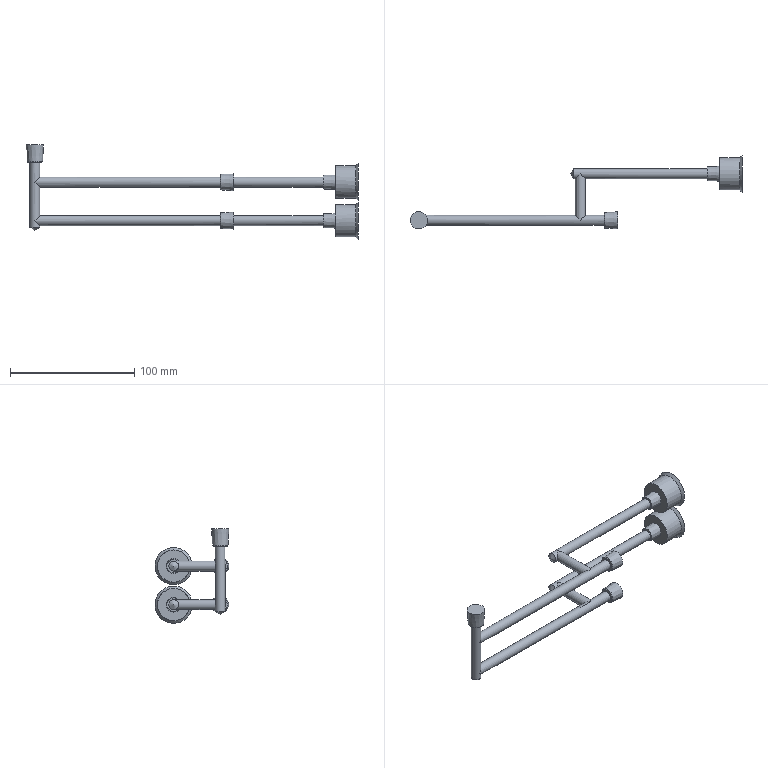Part | STEP file | COOLING-CAV_id202_x_t | 1 solid | 34 faces | box 267.068 x 59.568 x 76.003 mm | volume 57701 mm3 | cone 13 | plane 12 | cylinder 9 | commonest cylinder face diameters 8 x7 26 x2
STEP:
#1=CARTESIAN_POINT('',(200.,90.5,-11.));
#2=VERTEX_POINT('',#1);
#3=CARTESIAN_POINT('',(200.,75.5,-11.));
#4=DIRECTION('',(-1.,0.,0.));
#5=DIRECTION('',(0.,1.,0.));
#6=AXIS2_PLACEMENT_3D('',#3,#4,#5);
#7=CIRCLE('',#6,15.);
#8=EDGE_CURVE('',#2,#2,#7,.T.);
#9=ORIENTED_EDGE('',*,*,#8,.F.);
#10=EDGE_LOOP('',(#9));
#11=FACE_OUTER_BOUND('',#10,.T.);
#12=CARTESIAN_POINT('',(200.,75.5,-11.));
#13=DIRECTION('',(1.,0.,0.));
#14=DIRECTION('',(0.,0.,-1.));
#15=AXIS2_PLACEMENT_3D('',#12,#13,#14);
#16=PLANE('',#15);
#17=ADVANCED_FACE('',(#11),#16,.T.);
#18=ORIENTED_EDGE('',*,*,#8,.T.);
#19=EDGE_LOOP('',(#18));
#20=FACE_BOUND('',#19,.T.);
#21=CARTESIAN_POINT('',(198.,75.5,-24.));
#22=VERTEX_POINT('',#21);
#23=CARTESIAN_POINT('',(198.,75.5,-11.));
#24=DIRECTION('',(-1.,0.,0.));
#25=DIRECTION('',(0.,0.,-1.));
#26=AXIS2_PLACEMENT_3D('',#23,#24,#25);
#27=CIRCLE('',#26,13.);
#28=EDGE_CURVE('',#22,#22,#27,.T.);
#29=ORIENTED_EDGE('',*,*,#28,.F.);
#30=EDGE_LOOP('',(#29));
#31=FACE_BOUND('',#30,.T.);
#32=CARTESIAN_POINT('',(200.,75.5,-11.));
#33=DIRECTION('',(1.,0.,0.));
#34=DIRECTION('',(0.,1.,0.));
#35=AXIS2_PLACEMENT_3D('',#32,#33,#34);
#36=CONICAL_SURFACE('',#35,15.,45.);
#37=ADVANCED_FACE('',(#20,#31),#36,.T.);
#38=CARTESIAN_POINT('',(200.,90.5,20.));
#39=VERTEX_POINT('',#38);
#40=CARTESIAN_POINT('',(200.,75.5,20.));
#41=DIRECTION('',(-1.,0.,0.));
#42=DIRECTION('',(0.,1.,0.));
#43=AXIS2_PLACEMENT_3D('',#40,#41,#42);
#44=CIRCLE('',#43,15.);
#45=EDGE_CURVE('',#39,#39,#44,.T.);
#46=ORIENTED_EDGE('',*,*,#45,.F.);
#47=EDGE_LOOP('',(#46));
#48=FACE_OUTER_BOUND('',#47,.T.);
#49=CARTESIAN_POINT('',(200.,75.5,20.));
#50=DIRECTION('',(-1.,0.,0.));
#51=DIRECTION('',(0.,0.,1.));
#52=AXIS2_PLACEMENT_3D('',#49,#50,#51);
#53=PLANE('',#52);
#54=ADVANCED_FACE('',(#48),#53,.F.);
#55=ORIENTED_EDGE('',*,*,#28,.T.);
#56=EDGE_LOOP('',(#55));
#57=FACE_BOUND('',#56,.T.);
#58=CARTESIAN_POINT('',(182.001,75.5,-24.));
#59=VERTEX_POINT('',#58);
#60=CARTESIAN_POINT('',(182.001,75.5,-11.));
#61=DIRECTION('',(1.,0.,0.));
#62=DIRECTION('',(0.,0.,-1.));
#63=AXIS2_PLACEMENT_3D('',#60,#61,#62);
#64=CIRCLE('',#63,13.);
#65=EDGE_CURVE('',#59,#59,#64,.T.);
#66=ORIENTED_EDGE('',*,*,#65,.T.);
#67=EDGE_LOOP('',(#66));
#68=FACE_BOUND('',#67,.T.);
#69=CARTESIAN_POINT('',(206.888,75.5,-11.));
#70=DIRECTION('',(1.,0.,0.));
#71=DIRECTION('',(0.,0.,-1.));
#72=AXIS2_PLACEMENT_3D('',#69,#70,#71);
#73=CYLINDRICAL_SURFACE('',#72,13.);
#74=ADVANCED_FACE('',(#57,#68),#73,.T.);
#75=CARTESIAN_POINT('',(198.,75.5,33.));
#76=VERTEX_POINT('',#75);
#77=CARTESIAN_POINT('',(198.,75.5,20.));
#78=DIRECTION('',(-1.,0.,0.));
#79=DIRECTION('',(0.,0.,1.));
#80=AXIS2_PLACEMENT_3D('',#77,#78,#79);
#81=CIRCLE('',#80,13.);
#82=EDGE_CURVE('',#76,#76,#81,.T.);
#83=ORIENTED_EDGE('',*,*,#82,.F.);
#84=EDGE_LOOP('',(#83));
#85=FACE_BOUND('',#84,.T.);
#86=ORIENTED_EDGE('',*,*,#45,.T.);
#87=EDGE_LOOP('',(#86));
#88=FACE_BOUND('',#87,.T.);
#89=CARTESIAN_POINT('',(200.,75.5,20.));
#90=DIRECTION('',(1.,0.,0.));
#91=DIRECTION('',(0.,1.,0.));
#92=AXIS2_PLACEMENT_3D('',#89,#90,#91);
#93=CONICAL_SURFACE('',#92,15.,45.);
#94=ADVANCED_FACE('',(#85,#88),#93,.T.);
#95=CARTESIAN_POINT('',(182.001,75.5,-16.955));
#96=VERTEX_POINT('',#95);
#97=CARTESIAN_POINT('',(182.001,75.5,-11.));
#98=DIRECTION('',(-1.,0.,0.));
#99=DIRECTION('',(0.,0.,-1.));
#100=AXIS2_PLACEMENT_3D('',#97,#98,#99);
#101=CIRCLE('',#100,5.955);
#102=EDGE_CURVE('',#96,#96,#101,.T.);
#103=ORIENTED_EDGE('',*,*,#102,.F.);
#104=EDGE_LOOP('',(#103));
#105=FACE_BOUND('',#104,.T.);
#106=ORIENTED_EDGE('',*,*,#65,.F.);
#107=EDGE_LOOP('',(#106));
#108=FACE_BOUND('',#107,.T.);
#109=CARTESIAN_POINT('',(182.001,75.5,-11.));
#110=DIRECTION('',(1.,0.,0.));
#111=DIRECTION('',(0.,0.,-1.));
#112=AXIS2_PLACEMENT_3D('',#109,#110,#111);
#113=PLANE('',#112);
#114=ADVANCED_FACE('',(#105,#108),#113,.F.);
#115=CARTESIAN_POINT('',(182.001,75.5,33.));
#116=VERTEX_POINT('',#115);
#117=CARTESIAN_POINT('',(182.001,75.5,20.));
#118=DIRECTION('',(-1.,0.,0.));
#119=DIRECTION('',(0.,0.,1.));
#120=AXIS2_PLACEMENT_3D('',#117,#118,#119);
#121=CIRCLE('',#120,13.);
#122=EDGE_CURVE('',#116,#116,#121,.T.);
#123=ORIENTED_EDGE('',*,*,#122,.F.);
#124=EDGE_LOOP('',(#123));
#125=FACE_BOUND('',#124,.T.);
#126=ORIENTED_EDGE('',*,*,#82,.T.);
#127=EDGE_LOOP('',(#126));
#128=FACE_BOUND('',#127,.T.);
#129=CARTESIAN_POINT('',(55.348,75.5,20.));
#130=DIRECTION('',(-1.,0.,0.));
#131=DIRECTION('',(0.,0.,1.));
#132=AXIS2_PLACEMENT_3D('',#129,#130,#131);
#133=CYLINDRICAL_SURFACE('',#132,13.);
#134=ADVANCED_FACE('',(#125,#128),#133,.T.);
#135=ORIENTED_EDGE('',*,*,#102,.T.);
#136=EDGE_LOOP('',(#135));
#137=FACE_BOUND('',#136,.T.);
#138=CARTESIAN_POINT('',(172.001,75.5,-16.5));
#139=VERTEX_POINT('',#138);
#140=CARTESIAN_POINT('',(172.001,75.5,-11.));
#141=DIRECTION('',(1.,0.,0.));
#142=DIRECTION('',(0.,0.,-1.));
#143=AXIS2_PLACEMENT_3D('',#140,#141,#142);
#144=CIRCLE('',#143,5.5);
#145=EDGE_CURVE('',#139,#139,#144,.T.);
#146=ORIENTED_EDGE('',*,*,#145,.T.);
#147=EDGE_LOOP('',(#146));
#148=FACE_BOUND('',#147,.T.);
#149=CARTESIAN_POINT('',(182.001,75.5,-11.));
#150=DIRECTION('',(1.,0.,0.));
#151=DIRECTION('',(0.,0.,-1.));
#152=AXIS2_PLACEMENT_3D('',#149,#150,#151);
#153=CONICAL_SURFACE('',#152,5.955,2.603);
#154=ADVANCED_FACE('',(#137,#148),#153,.T.);
#155=CARTESIAN_POINT('',(182.001,75.5,14.045));
#156=VERTEX_POINT('',#155);
#157=CARTESIAN_POINT('',(182.001,75.5,20.));
#158=DIRECTION('',(-1.,0.,0.));
#159=DIRECTION('',(0.,0.,-1.));
#160=AXIS2_PLACEMENT_3D('',#157,#158,#159);
#161=CIRCLE('',#160,5.955);
#162=EDGE_CURVE('',#156,#156,#161,.T.);
#163=ORIENTED_EDGE('',*,*,#162,.F.);
#164=EDGE_LOOP('',(#163));
#165=FACE_BOUND('',#164,.T.);
#166=ORIENTED_EDGE('',*,*,#122,.T.);
#167=EDGE_LOOP('',(#166));
#168=FACE_BOUND('',#167,.T.);
#169=CARTESIAN_POINT('',(182.001,75.5,20.));
#170=DIRECTION('',(-1.,0.,0.));
#171=DIRECTION('',(0.,0.,1.));
#172=AXIS2_PLACEMENT_3D('',#169,#170,#171);
#173=PLANE('',#172);
#174=ADVANCED_FACE('',(#165,#168),#173,.T.);
#175=CARTESIAN_POINT('',(100.,44.884,-11.));
#176=VERTEX_POINT('',#175);
#177=CARTESIAN_POINT('',(100.,38.,-11.));
#178=DIRECTION('',(-1.,0.,0.));
#179=DIRECTION('',(0.,1.,0.));
#180=AXIS2_PLACEMENT_3D('',#177,#178,#179);
#181=CIRCLE('',#180,6.884);
#182=EDGE_CURVE('',#176,#176,#181,.T.);
#183=ORIENTED_EDGE('',*,*,#182,.F.);
#184=EDGE_LOOP('',(#183));
#185=FACE_OUTER_BOUND('',#184,.T.);
#186=CARTESIAN_POINT('',(100.,38.,-11.));
#187=DIRECTION('',(1.,0.,0.));
#188=DIRECTION('',(0.,0.,-1.));
#189=AXIS2_PLACEMENT_3D('',#186,#187,#188);
#190=PLANE('',#189);
#191=ADVANCED_FACE('',(#185),#190,.T.);
#192=CARTESIAN_POINT('',(172.001,75.5,-15.));
#193=VERTEX_POINT('',#192);
#194=CARTESIAN_POINT('',(172.001,75.5,-11.));
#195=DIRECTION('',(-1.,0.,0.));
#196=DIRECTION('',(0.,0.,-1.));
#197=AXIS2_PLACEMENT_3D('',#194,#195,#196);
#198=CIRCLE('',#197,4.);
#199=EDGE_CURVE('',#193,#193,#198,.T.);
#200=ORIENTED_EDGE('',*,*,#199,.F.);
#201=EDGE_LOOP('',(#200));
#202=FACE_BOUND('',#201,.T.);
#203=ORIENTED_EDGE('',*,*,#145,.F.);
#204=EDGE_LOOP('',(#203));
#205=FACE_BOUND('',#204,.T.);
#206=CARTESIAN_POINT('',(172.001,75.5,-11.));
#207=DIRECTION('',(1.,0.,0.));
#208=DIRECTION('',(0.,0.,-1.));
#209=AXIS2_PLACEMENT_3D('',#206,#207,#208);
#210=PLANE('',#209);
#211=ADVANCED_FACE('',(#202,#205),#210,.F.);
#212=CARTESIAN_POINT('',(64.459,75.5,-15.));
#213=VERTEX_POINT('',#212);
#214=CARTESIAN_POINT('',(64.459,75.5,-11.));
#215=DIRECTION('',(1.,0.,0.));
#216=DIRECTION('',(0.,0.,-1.));
#217=AXIS2_PLACEMENT_3D('',#214,#215,#216);
#218=CIRCLE('',#217,4.);
#219=EDGE_CURVE('',#213,#213,#218,.T.);
#220=ORIENTED_EDGE('',*,*,#219,.F.);
#221=EDGE_LOOP('',(#220));
#222=FACE_BOUND('',#221,.T.);
#223=CARTESIAN_POINT('',(62.236,75.5,-11.));
#224=VERTEX_POINT('',#223);
#225=VERTEX_LOOP('',#224);
#226=FACE_BOUND('',#225,.T.);
#227=CARTESIAN_POINT('',(64.459,75.5,-11.));
#228=DIRECTION('',(1.,0.,0.));
#229=DIRECTION('',(0.,0.,-1.));
#230=AXIS2_PLACEMENT_3D('',#227,#228,#229);
#231=CONICAL_SURFACE('',#230,4.,60.942);
#232=ADVANCED_FACE('',(#222,#226),#231,.T.);
#233=CARTESIAN_POINT('',(172.001,75.5,14.5));
#234=VERTEX_POINT('',#233);
#235=CARTESIAN_POINT('',(172.001,75.5,20.));
#236=DIRECTION('',(-1.,0.,0.));
#237=DIRECTION('',(0.,0.,-1.));
#238=AXIS2_PLACEMENT_3D('',#235,#236,#237);
#239=CIRCLE('',#238,5.5);
#240=EDGE_CURVE('',#234,#234,#239,.T.);
#241=ORIENTED_EDGE('',*,*,#240,.F.);
#242=EDGE_LOOP('',(#241));
#243=FACE_BOUND('',#242,.T.);
#244=ORIENTED_EDGE('',*,*,#162,.T.);
#245=EDGE_LOOP('',(#244));
#246=FACE_BOUND('',#245,.T.);
#247=CARTESIAN_POINT('',(182.001,75.5,20.));
#248=DIRECTION('',(1.,0.,0.));
#249=DIRECTION('',(0.,0.,-1.));
#250=AXIS2_PLACEMENT_3D('',#247,#248,#249);
#251=CONICAL_SURFACE('',#250,5.955,2.603);
#252=ADVANCED_FACE('',(#243,#246),#251,.T.);
#253=CARTESIAN_POINT('',(-52.932,38.,50.003));
#254=VERTEX_POINT('',#253);
#255=CARTESIAN_POINT('',(-60.,38.,50.003));
#256=DIRECTION('',(0.,0.,-1.));
#257=DIRECTION('',(1.,0.,0.));
#258=AXIS2_PLACEMENT_3D('',#255,#256,#257);
#259=CIRCLE('',#258,7.068);
#260=EDGE_CURVE('',#254,#254,#259,.T.);
#261=ORIENTED_EDGE('',*,*,#260,.F.);
#262=EDGE_LOOP('',(#261));
#263=FACE_OUTER_BOUND('',#262,.T.);
#264=CARTESIAN_POINT('',(-60.,38.,50.003));
#265=DIRECTION('',(0.,0.,1.));
#266=DIRECTION('',(1.,0.,0.));
#267=AXIS2_PLACEMENT_3D('',#264,#265,#266);
#268=PLANE('',#267);
#269=ADVANCED_FACE('',(#263),#268,.T.);
#270=ORIENTED_EDGE('',*,*,#182,.T.);
#271=EDGE_LOOP('',(#270));
#272=FACE_BOUND('',#271,.T.);
#273=CARTESIAN_POINT('',(89.5,38.,-4.758));
#274=VERTEX_POINT('',#273);
#275=CARTESIAN_POINT('',(89.5,38.,-11.));
#276=DIRECTION('',(-1.,0.,0.));
#277=DIRECTION('',(0.,0.,1.));
#278=AXIS2_PLACEMENT_3D('',#275,#276,#277);
#279=CIRCLE('',#278,6.242);
#280=EDGE_CURVE('',#274,#274,#279,.T.);
#281=ORIENTED_EDGE('',*,*,#280,.F.);
#282=EDGE_LOOP('',(#281));
#283=FACE_BOUND('',#282,.T.);
#284=CARTESIAN_POINT('',(100.,38.,-11.));
#285=DIRECTION('',(1.,0.,0.));
#286=DIRECTION('',(0.,1.,0.));
#287=AXIS2_PLACEMENT_3D('',#284,#285,#286);
#288=CONICAL_SURFACE('',#287,6.884,3.5);
#289=ADVANCED_FACE('',(#272,#283),#288,.T.);
#290=ORIENTED_EDGE('',*,*,#199,.T.);
#291=EDGE_LOOP('',(#290));
#292=FACE_BOUND('',#291,.T.);
#293=ORIENTED_EDGE('',*,*,#219,.T.);
#294=EDGE_LOOP('',(#293));
#295=FACE_BOUND('',#294,.T.);
#296=CARTESIAN_POINT('',(70.,75.5,-7.));
#297=VERTEX_POINT('',#296);
#298=CARTESIAN_POINT('',(70.,75.5,-15.));
#299=VERTEX_POINT('',#298);
#300=CARTESIAN_POINT('',(70.,75.5,-11.));
#301=DIRECTION('',(0.7071,-0.7071,0.));
#302=DIRECTION('',(0.7071,0.7071,0.));
#303=AXIS2_PLACEMENT_3D('',#300,#301,#302);
#304=ELLIPSE('',#303,5.657,4.);
#305=EDGE_CURVE('',#297,#299,#304,.T.);
#306=ORIENTED_EDGE('',*,*,#305,.F.);
#307=CARTESIAN_POINT('',(70.,75.5,-11.));
#308=DIRECTION('',(-0.7071,-0.7071,0.));
#309=DIRECTION('',(0.7071,-0.7071,0.));
#310=AXIS2_PLACEMENT_3D('',#307,#308,#309);
#311=ELLIPSE('',#310,5.657,4.);
#312=EDGE_CURVE('',#299,#297,#311,.T.);
#313=ORIENTED_EDGE('',*,*,#312,.F.);
#314=EDGE_LOOP('',(#306,#313));
#315=FACE_BOUND('',#314,.T.);
#316=CARTESIAN_POINT('',(206.888,75.5,-11.));
#317=DIRECTION('',(1.,0.,0.));
#318=DIRECTION('',(0.,0.,-1.));
#319=AXIS2_PLACEMENT_3D('',#316,#317,#318);
#320=CYLINDRICAL_SURFACE('',#319,4.);
#321=ADVANCED_FACE('',(#292,#295,#315),#320,.T.);
#322=CARTESIAN_POINT('',(100.,38.,13.116));
#323=VERTEX_POINT('',#322);
#324=CARTESIAN_POINT('',(100.,38.,20.));
#325=DIRECTION('',(-1.,0.,0.));
#326=DIRECTION('',(0.,0.,-1.));
#327=AXIS2_PLACEMENT_3D('',#324,#325,#326);
#328=CIRCLE('',#327,6.884);
#329=EDGE_CURVE('',#323,#323,#328,.T.);
#330=ORIENTED_EDGE('',*,*,#329,.F.);
#331=EDGE_LOOP('',(#330));
#332=FACE_OUTER_BOUND('',#331,.T.);
#333=CARTESIAN_POINT('',(100.,38.,20.));
#334=DIRECTION('',(-1.,0.,0.));
#335=DIRECTION('',(0.,0.,1.));
#336=AXIS2_PLACEMENT_3D('',#333,#334,#335);
#337=PLANE('',#336);
#338=ADVANCED_FACE('',(#332),#337,.F.);
#339=CARTESIAN_POINT('',(62.236,75.5,20.));
#340=VERTEX_POINT('',#339);
#341=VERTEX_LOOP('',#340);
#342=FACE_BOUND('',#341,.T.);
#343=CARTESIAN_POINT('',(64.459,75.5,24.));
#344=VERTEX_POINT('',#343);
#345=CARTESIAN_POINT('',(64.459,75.5,20.));
#346=DIRECTION('',(1.,0.,0.));
#347=DIRECTION('',(0.,0.,1.));
#348=AXIS2_PLACEMENT_3D('',#345,#346,#347);
#349=CIRCLE('',#348,4.);
#350=EDGE_CURVE('',#344,#344,#349,.T.);
#351=ORIENTED_EDGE('',*,*,#350,.F.);
#352=EDGE_LOOP('',(#351));
#353=FACE_BOUND('',#352,.T.);
#354=CARTESIAN_POINT('',(64.459,75.5,20.));
#355=DIRECTION('',(1.,0.,0.));
#356=DIRECTION('',(0.,0.,-1.));
#357=AXIS2_PLACEMENT_3D('',#354,#355,#356);
#358=CONICAL_SURFACE('',#357,4.,60.942);
#359=ADVANCED_FACE('',(#342,#353),#358,.T.);
#360=CARTESIAN_POINT('',(172.001,75.5,24.));
#361=VERTEX_POINT('',#360);
#362=CARTESIAN_POINT('',(172.001,75.5,20.));
#363=DIRECTION('',(-1.,0.,0.));
#364=DIRECTION('',(0.,0.,1.));
#365=AXIS2_PLACEMENT_3D('',#362,#363,#364);
#366=CIRCLE('',#365,4.);
#367=EDGE_CURVE('',#361,#361,#366,.T.);
#368=ORIENTED_EDGE('',*,*,#367,.F.);
#369=EDGE_LOOP('',(#368));
#370=FACE_BOUND('',#369,.T.);
#371=ORIENTED_EDGE('',*,*,#240,.T.);
#372=EDGE_LOOP('',(#371));
#373=FACE_BOUND('',#372,.T.);
#374=CARTESIAN_POINT('',(172.001,75.5,20.));
#375=DIRECTION('',(-1.,0.,0.));
#376=DIRECTION('',(0.,0.,1.));
#377=AXIS2_PLACEMENT_3D('',#374,#375,#376);
#378=PLANE('',#377);
#379=ADVANCED_FACE('',(#370,#373),#378,.T.);
#380=ORIENTED_EDGE('',*,*,#260,.T.);
#381=EDGE_LOOP('',(#380));
#382=FACE_BOUND('',#381,.T.);
#383=CARTESIAN_POINT('',(-66.242,38.,36.503));
#384=VERTEX_POINT('',#383);
#385=CARTESIAN_POINT('',(-60.,38.,36.503));
#386=DIRECTION('',(0.,0.,-1.));
#387=DIRECTION('',(-1.,0.,0.));
#388=AXIS2_PLACEMENT_3D('',#385,#386,#387);
#389=CIRCLE('',#388,6.242);
#390=EDGE_CURVE('',#384,#384,#389,.T.);
#391=ORIENTED_EDGE('',*,*,#390,.F.);
#392=EDGE_LOOP('',(#391));
#393=FACE_BOUND('',#392,.T.);
#394=CARTESIAN_POINT('',(-60.,38.,50.003));
#395=DIRECTION('',(0.,0.,1.));
#396=DIRECTION('',(1.,0.,0.));
#397=AXIS2_PLACEMENT_3D('',#394,#395,#396);
#398=CONICAL_SURFACE('',#397,7.068,3.5);
#399=ADVANCED_FACE('',(#382,#393),#398,.T.);
#400=ORIENTED_EDGE('',*,*,#280,.T.);
#401=EDGE_LOOP('',(#400));
#402=FACE_BOUND('',#401,.T.);
#403=CARTESIAN_POINT('',(89.,38.,-16.742));
#404=VERTEX_POINT('',#403);
#405=CARTESIAN_POINT('',(89.,38.,-11.));
#406=DIRECTION('',(1.,0.,0.));
#407=DIRECTION('',(0.,0.,-1.));
#408=AXIS2_PLACEMENT_3D('',#405,#406,#407);
#409=CIRCLE('',#408,5.742);
#410=EDGE_CURVE('',#404,#404,#409,.T.);
#411=ORIENTED_EDGE('',*,*,#410,.T.);
#412=EDGE_LOOP('',(#411));
#413=FACE_BOUND('',#412,.T.);
#414=CARTESIAN_POINT('',(89.5,38.,-11.));
#415=DIRECTION('',(1.,0.,0.));
#416=DIRECTION('',(0.,0.,-1.));
#417=AXIS2_PLACEMENT_3D('',#414,#415,#416);
#418=CONICAL_SURFACE('',#417,6.242,45.);
#419=ADVANCED_FACE('',(#402,#413),#418,.T.);
#420=CARTESIAN_POINT('',(70.,38.,-7.));
#421=VERTEX_POINT('',#420);
#422=CARTESIAN_POINT('',(70.,38.,-15.));
#423=VERTEX_POINT('',#422);
#424=CARTESIAN_POINT('',(70.,38.,-11.));
#425=DIRECTION('',(-0.7071,-0.7071,0.));
#426=DIRECTION('',(0.7071,-0.7071,0.));
#427=AXIS2_PLACEMENT_3D('',#424,#425,#426);
#428=ELLIPSE('',#427,5.657,4.);
#429=EDGE_CURVE('',#421,#423,#428,.T.);
#430=ORIENTED_EDGE('',*,*,#429,.F.);
#431=CARTESIAN_POINT('',(70.,38.,-11.));
#432=DIRECTION('',(0.7071,-0.7071,0.));
#433=DIRECTION('',(0.7071,0.7071,0.));
#434=AXIS2_PLACEMENT_3D('',#431,#432,#433);
#435=ELLIPSE('',#434,5.657,4.);
#436=EDGE_CURVE('',#423,#421,#435,.T.);
#437=ORIENTED_EDGE('',*,*,#436,.F.);
#438=EDGE_LOOP('',(#430,#437));
#439=FACE_BOUND('',#438,.T.);
#440=ORIENTED_EDGE('',*,*,#312,.T.);
#441=ORIENTED_EDGE('',*,*,#305,.T.);
#442=EDGE_LOOP('',(#440,#441));
#443=FACE_BOUND('',#442,.T.);
#444=CARTESIAN_POINT('',(70.,38.,-11.));
#445=DIRECTION('',(0.,-1.,0.));
#446=DIRECTION('',(0.,0.,-1.));
#447=AXIS2_PLACEMENT_3D('',#444,#445,#446);
#448=CYLINDRICAL_SURFACE('',#447,4.);
#449=ADVANCED_FACE('',(#439,#443),#448,.T.);
#450=CARTESIAN_POINT('',(89.5,38.,26.242));
#451=VERTEX_POINT('',#450);
#452=CARTESIAN_POINT('',(89.5,38.,20.));
#453=DIRECTION('',(-1.,0.,0.));
#454=DIRECTION('',(0.,0.,1.));
#455=AXIS2_PLACEMENT_3D('',#452,#453,#454);
#456=CIRCLE('',#455,6.242);
#457=EDGE_CURVE('',#451,#451,#456,.T.);
#458=ORIENTED_EDGE('',*,*,#457,.F.);
#459=EDGE_LOOP('',(#458));
#460=FACE_BOUND('',#459,.T.);
#461=ORIENTED_EDGE('',*,*,#329,.T.);
#462=EDGE_LOOP('',(#461));
#463=FACE_BOUND('',#462,.T.);
#464=CARTESIAN_POINT('',(100.,38.,20.));
#465=DIRECTION('',(1.,0.,0.));
#466=DIRECTION('',(0.,0.,-1.));
#467=AXIS2_PLACEMENT_3D('',#464,#465,#466);
#468=CONICAL_SURFACE('',#467,6.884,3.5);
#469=ADVANCED_FACE('',(#460,#463),#468,.T.);
#470=ORIENTED_EDGE('',*,*,#350,.T.);
#471=EDGE_LOOP('',(#470));
#472=FACE_BOUND('',#471,.T.);
#473=ORIENTED_EDGE('',*,*,#367,.T.);
#474=EDGE_LOOP('',(#473));
#475=FACE_BOUND('',#474,.T.);
#476=CARTESIAN_POINT('',(70.,75.5,24.));
#477=VERTEX_POINT('',#476);
#478=CARTESIAN_POINT('',(70.,75.5,16.));
#479=VERTEX_POINT('',#478);
#480=CARTESIAN_POINT('',(70.,75.5,20.));
#481=DIRECTION('',(0.7071,-0.7071,0.));
#482=DIRECTION('',(-0.7071,-0.7071,0.));
#483=AXIS2_PLACEMENT_3D('',#480,#481,#482);
#484=ELLIPSE('',#483,5.657,4.);
#485=EDGE_CURVE('',#477,#479,#484,.T.);
#486=ORIENTED_EDGE('',*,*,#485,.F.);
#487=CARTESIAN_POINT('',(70.,75.5,20.));
#488=DIRECTION('',(-0.7071,-0.7071,0.));
#489=DIRECTION('',(0.7071,-0.7071,0.));
#490=AXIS2_PLACEMENT_3D('',#487,#488,#489);
#491=ELLIPSE('',#490,5.657,4.);
#492=EDGE_CURVE('',#479,#477,#491,.T.);
#493=ORIENTED_EDGE('',*,*,#492,.F.);
#494=EDGE_LOOP('',(#486,#493));
#495=FACE_BOUND('',#494,.T.);
#496=CARTESIAN_POINT('',(55.348,75.5,20.));
#497=DIRECTION('',(-1.,0.,0.));
#498=DIRECTION('',(0.,0.,1.));
#499=AXIS2_PLACEMENT_3D('',#496,#497,#498);
#500=CYLINDRICAL_SURFACE('',#499,4.);
#501=ADVANCED_FACE('',(#472,#475,#495),#500,.T.);
#502=ORIENTED_EDGE('',*,*,#390,.T.);
#503=EDGE_LOOP('',(#502));
#504=FACE_BOUND('',#503,.T.);
#505=CARTESIAN_POINT('',(-54.258,38.,36.003));
#506=VERTEX_POINT('',#505);
#507=CARTESIAN_POINT('',(-60.,38.,36.003));
#508=DIRECTION('',(0.,0.,1.));
#509=DIRECTION('',(1.,0.,0.));
#510=AXIS2_PLACEMENT_3D('',#507,#508,#509);
#511=CIRCLE('',#510,5.742);
#512=EDGE_CURVE('',#506,#506,#511,.T.);
#513=ORIENTED_EDGE('',*,*,#512,.T.);
#514=EDGE_LOOP('',(#513));
#515=FACE_BOUND('',#514,.T.);
#516=CARTESIAN_POINT('',(-60.,38.,36.503));
#517=DIRECTION('',(0.,0.,1.));
#518=DIRECTION('',(1.,0.,0.));
#519=AXIS2_PLACEMENT_3D('',#516,#517,#518);
#520=CONICAL_SURFACE('',#519,6.242,45.);
#521=ADVANCED_FACE('',(#504,#515),#520,.T.);
#522=CARTESIAN_POINT('',(89.,38.,-15.));
#523=VERTEX_POINT('',#522);
#524=CARTESIAN_POINT('',(89.,38.,-11.));
#525=DIRECTION('',(-1.,0.,0.));
#526=DIRECTION('',(0.,0.,-1.));
#527=AXIS2_PLACEMENT_3D('',#524,#525,#526);
#528=CIRCLE('',#527,4.);
#529=EDGE_CURVE('',#523,#523,#528,.T.);
#530=ORIENTED_EDGE('',*,*,#529,.F.);
#531=EDGE_LOOP('',(#530));
#532=FACE_BOUND('',#531,.T.);
#533=ORIENTED_EDGE('',*,*,#410,.F.);
#534=EDGE_LOOP('',(#533));
#535=FACE_BOUND('',#534,.T.);
#536=CARTESIAN_POINT('',(89.,38.,-11.));
#537=DIRECTION('',(1.,0.,0.));
#538=DIRECTION('',(0.,0.,-1.));
#539=AXIS2_PLACEMENT_3D('',#536,#537,#538);
#540=PLANE('',#539);
#541=ADVANCED_FACE('',(#532,#535),#540,.F.);
#542=CARTESIAN_POINT('',(89.,38.,14.258));
#543=VERTEX_POINT('',#542);
#544=CARTESIAN_POINT('',(89.,38.,20.));
#545=DIRECTION('',(-1.,0.,0.));
#546=DIRECTION('',(0.,0.,-1.));
#547=AXIS2_PLACEMENT_3D('',#544,#545,#546);
#548=CIRCLE('',#547,5.742);
#549=EDGE_CURVE('',#543,#543,#548,.T.);
#550=ORIENTED_EDGE('',*,*,#549,.F.);
#551=EDGE_LOOP('',(#550));
#552=FACE_BOUND('',#551,.T.);
#553=ORIENTED_EDGE('',*,*,#457,.T.);
#554=EDGE_LOOP('',(#553));
#555=FACE_BOUND('',#554,.T.);
#556=CARTESIAN_POINT('',(89.5,38.,20.));
#557=DIRECTION('',(1.,0.,0.));
#558=DIRECTION('',(0.,0.,-1.));
#559=AXIS2_PLACEMENT_3D('',#556,#557,#558);
#560=CONICAL_SURFACE('',#559,6.242,45.);
#561=ADVANCED_FACE('',(#552,#555),#560,.T.);
#562=ORIENTED_EDGE('',*,*,#492,.T.);
#563=ORIENTED_EDGE('',*,*,#485,.T.);
#564=EDGE_LOOP('',(#562,#563));
#565=FACE_BOUND('',#564,.T.);
#566=CARTESIAN_POINT('',(70.,38.,16.));
#567=VERTEX_POINT('',#566);
#568=CARTESIAN_POINT('',(70.,38.,24.));
#569=VERTEX_POINT('',#568);
#570=CARTESIAN_POINT('',(70.,38.,20.));
#571=DIRECTION('',(0.7071,-0.7071,0.));
#572=DIRECTION('',(-0.7071,-0.7071,0.));
#573=AXIS2_PLACEMENT_3D('',#570,#571,#572);
#574=ELLIPSE('',#573,5.657,4.);
#575=EDGE_CURVE('',#567,#569,#574,.T.);
#576=ORIENTED_EDGE('',*,*,#575,.F.);
#577=CARTESIAN_POINT('',(70.,38.,20.));
#578=DIRECTION('',(-0.7071,-0.7071,0.));
#579=DIRECTION('',(0.7071,-0.7071,0.));
#580=AXIS2_PLACEMENT_3D('',#577,#578,#579);
#581=ELLIPSE('',#580,5.657,4.);
#582=EDGE_CURVE('',#569,#567,#581,.T.);
#583=ORIENTED_EDGE('',*,*,#582,.F.);
#584=EDGE_LOOP('',(#576,#583));
#585=FACE_BOUND('',#584,.T.);
#586=CARTESIAN_POINT('',(70.,38.,20.));
#587=DIRECTION('',(0.,-1.,0.));
#588=DIRECTION('',(0.,0.,-1.));
#589=AXIS2_PLACEMENT_3D('',#586,#587,#588);
#590=CYLINDRICAL_SURFACE('',#589,4.);
#591=ADVANCED_FACE('',(#565,#585),#590,.T.);
#592=CARTESIAN_POINT('',(-56.,38.,36.003));
#593=VERTEX_POINT('',#592);
#594=CARTESIAN_POINT('',(-60.,38.,36.003));
#595=DIRECTION('',(0.,0.,-1.));
#596=DIRECTION('',(1.,0.,0.));
#597=AXIS2_PLACEMENT_3D('',#594,#595,#596);
#598=CIRCLE('',#597,4.);
#599=EDGE_CURVE('',#593,#593,#598,.T.);
#600=ORIENTED_EDGE('',*,*,#599,.F.);
#601=EDGE_LOOP('',(#600));
#602=FACE_BOUND('',#601,.T.);
#603=ORIENTED_EDGE('',*,*,#512,.F.);
#604=EDGE_LOOP('',(#603));
#605=FACE_BOUND('',#604,.T.);
#606=CARTESIAN_POINT('',(-60.,38.,36.003));
#607=DIRECTION('',(0.,0.,1.));
#608=DIRECTION('',(1.,0.,0.));
#609=AXIS2_PLACEMENT_3D('',#606,#607,#608);
#610=PLANE('',#609);
#611=ADVANCED_FACE('',(#602,#605),#610,.F.);
#612=CARTESIAN_POINT('',(-56.,38.,-16.541));
#613=VERTEX_POINT('',#612);
#614=CARTESIAN_POINT('',(-60.,38.,-16.541));
#615=DIRECTION('',(0.,0.,1.));
#616=DIRECTION('',(1.,0.,0.));
#617=AXIS2_PLACEMENT_3D('',#614,#615,#616);
#618=CIRCLE('',#617,4.);
#619=EDGE_CURVE('',#613,#613,#618,.T.);
#620=ORIENTED_EDGE('',*,*,#619,.F.);
#621=EDGE_LOOP('',(#620));
#622=FACE_BOUND('',#621,.T.);
#623=CARTESIAN_POINT('',(-60.,38.,-18.764));
#624=VERTEX_POINT('',#623);
#625=VERTEX_LOOP('',#624);
#626=FACE_BOUND('',#625,.T.);
#627=CARTESIAN_POINT('',(-60.,38.,-16.541));
#628=DIRECTION('',(0.,0.,1.));
#629=DIRECTION('',(1.,0.,0.));
#630=AXIS2_PLACEMENT_3D('',#627,#628,#629);
#631=CONICAL_SURFACE('',#630,4.,60.942);
#632=ADVANCED_FACE('',(#622,#626),#631,.T.);
#633=ORIENTED_EDGE('',*,*,#429,.T.);
#634=ORIENTED_EDGE('',*,*,#436,.T.);
#635=EDGE_LOOP('',(#633,#634));
#636=FACE_BOUND('',#635,.T.);
#637=ORIENTED_EDGE('',*,*,#529,.T.);
#638=EDGE_LOOP('',(#637));
#639=FACE_BOUND('',#638,.T.);
#640=CARTESIAN_POINT('',(-60.,42.,-11.));
#641=VERTEX_POINT('',#640);
#642=CARTESIAN_POINT('',(-60.,34.,-11.));
#643=VERTEX_POINT('',#642);
#644=CARTESIAN_POINT('',(-60.,38.,-11.));
#645=DIRECTION('',(-0.7071,0.,-0.7071));
#646=DIRECTION('',(0.7071,0.,-0.7071));
#647=AXIS2_PLACEMENT_3D('',#644,#645,#646);
#648=ELLIPSE('',#647,5.657,4.);
#649=EDGE_CURVE('',#641,#643,#648,.T.);
#650=ORIENTED_EDGE('',*,*,#649,.F.);
#651=CARTESIAN_POINT('',(-60.,38.,-11.));
#652=DIRECTION('',(-0.7071,0.,0.7071));
#653=DIRECTION('',(0.7071,0.,0.7071));
#654=AXIS2_PLACEMENT_3D('',#651,#652,#653);
#655=ELLIPSE('',#654,5.657,4.);
#656=EDGE_CURVE('',#643,#641,#655,.T.);
#657=ORIENTED_EDGE('',*,*,#656,.F.);
#658=EDGE_LOOP('',(#650,#657));
#659=FACE_BOUND('',#658,.T.);
#660=CARTESIAN_POINT('',(108.,38.,-11.));
#661=DIRECTION('',(1.,0.,0.));
#662=DIRECTION('',(0.,0.,-1.));
#663=AXIS2_PLACEMENT_3D('',#660,#661,#662);
#664=CYLINDRICAL_SURFACE('',#663,4.);
#665=ADVANCED_FACE('',(#636,#639,#659),#664,.T.);
#666=CARTESIAN_POINT('',(89.,38.,24.));
#667=VERTEX_POINT('',#666);
#668=CARTESIAN_POINT('',(89.,38.,20.));
#669=DIRECTION('',(-1.,0.,0.));
#670=DIRECTION('',(0.,0.,1.));
#671=AXIS2_PLACEMENT_3D('',#668,#669,#670);
#672=CIRCLE('',#671,4.);
#673=EDGE_CURVE('',#667,#667,#672,.T.);
#674=ORIENTED_EDGE('',*,*,#673,.F.);
#675=EDGE_LOOP('',(#674));
#676=FACE_BOUND('',#675,.T.);
#677=ORIENTED_EDGE('',*,*,#549,.T.);
#678=EDGE_LOOP('',(#677));
#679=FACE_BOUND('',#678,.T.);
#680=CARTESIAN_POINT('',(89.,38.,20.));
#681=DIRECTION('',(-1.,0.,0.));
#682=DIRECTION('',(0.,0.,1.));
#683=AXIS2_PLACEMENT_3D('',#680,#681,#682);
#684=PLANE('',#683);
#685=ADVANCED_FACE('',(#676,#679),#684,.T.);
#686=ORIENTED_EDGE('',*,*,#619,.T.);
#687=EDGE_LOOP('',(#686));
#688=FACE_BOUND('',#687,.T.);
#689=CARTESIAN_POINT('',(-60.,42.,20.));
#690=VERTEX_POINT('',#689);
#691=CARTESIAN_POINT('',(-60.,34.,20.));
#692=VERTEX_POINT('',#691);
#693=CARTESIAN_POINT('',(-60.,38.,20.));
#694=DIRECTION('',(0.7071,0.,-0.7071));
#695=DIRECTION('',(0.7071,0.,0.7071));
#696=AXIS2_PLACEMENT_3D('',#693,#694,#695);
#697=ELLIPSE('',#696,5.657,4.);
#698=EDGE_CURVE('',#690,#692,#697,.T.);
#699=ORIENTED_EDGE('',*,*,#698,.F.);
#700=CARTESIAN_POINT('',(-60.,38.,20.));
#701=DIRECTION('',(0.7071,0.,0.7071));
#702=DIRECTION('',(-0.7071,0.,0.7071));
#703=AXIS2_PLACEMENT_3D('',#700,#701,#702);
#704=ELLIPSE('',#703,5.657,4.);
#705=EDGE_CURVE('',#692,#690,#704,.T.);
#706=ORIENTED_EDGE('',*,*,#705,.F.);
#707=EDGE_LOOP('',(#699,#706));
#708=FACE_BOUND('',#707,.T.);
#709=ORIENTED_EDGE('',*,*,#599,.T.);
#710=EDGE_LOOP('',(#709));
#711=FACE_BOUND('',#710,.T.);
#712=ORIENTED_EDGE('',*,*,#649,.T.);
#713=ORIENTED_EDGE('',*,*,#656,.T.);
#714=EDGE_LOOP('',(#712,#713));
#715=FACE_BOUND('',#714,.T.);
#716=CARTESIAN_POINT('',(-60.,38.,50.291));
#717=DIRECTION('',(0.,0.,1.));
#718=DIRECTION('',(1.,0.,0.));
#719=AXIS2_PLACEMENT_3D('',#716,#717,#718);
#720=CYLINDRICAL_SURFACE('',#719,4.);
#721=ADVANCED_FACE('',(#688,#708,#711,#715),#720,.T.);
#722=ORIENTED_EDGE('',*,*,#582,.T.);
#723=ORIENTED_EDGE('',*,*,#575,.T.);
#724=EDGE_LOOP('',(#722,#723));
#725=FACE_BOUND('',#724,.T.);
#726=ORIENTED_EDGE('',*,*,#673,.T.);
#727=EDGE_LOOP('',(#726));
#728=FACE_BOUND('',#727,.T.);
#729=ORIENTED_EDGE('',*,*,#698,.T.);
#730=ORIENTED_EDGE('',*,*,#705,.T.);
#731=EDGE_LOOP('',(#729,#730));
#732=FACE_BOUND('',#731,.T.);
#733=CARTESIAN_POINT('',(-68.,38.,20.));
#734=DIRECTION('',(-1.,0.,0.));
#735=DIRECTION('',(0.,0.,1.));
#736=AXIS2_PLACEMENT_3D('',#733,#734,#735);
#737=CYLINDRICAL_SURFACE('',#736,4.);
#738=ADVANCED_FACE('',(#725,#728,#732),#737,.T.);
#739=CLOSED_SHELL('',(#17,#37,#54,#74,#94,#114,#134,#154,#174,#191,#211,#232,#252,#269,#289,#321,#338,#359,#379,#399,#419,#449,#469,#501,#521,#541,#561,#591,#611,#632,#665,#685,#721,#738));
#740=MANIFOLD_SOLID_BREP('',#739);
#741=(LENGTH_UNIT()NAMED_UNIT(*)SI_UNIT(.MILLI.,.METRE.));
#742=UNCERTAINTY_MEASURE_WITH_UNIT(LENGTH_MEASURE(0.00004123),#741,'','');
#743=(NAMED_UNIT(*)PLANE_ANGLE_UNIT()SI_UNIT($,.RADIAN.));
#744=PLANE_ANGLE_MEASURE_WITH_UNIT(PLANE_ANGLE_MEASURE(0.01745),#743);
#745=DIMENSIONAL_EXPONENTS(0.,0.,0.,0.,0.,0.,0.);
#746=(CONVERSION_BASED_UNIT('DEGREE',#744)NAMED_UNIT(#745)PLANE_ANGLE_UNIT());
#747=(NAMED_UNIT(*)SI_UNIT($,.STERADIAN.)SOLID_ANGLE_UNIT());
#748=(GEOMETRIC_REPRESENTATION_CONTEXT(3)GLOBAL_UNCERTAINTY_ASSIGNED_CONTEXT((#742))GLOBAL_UNIT_ASSIGNED_CONTEXT((#741,#746,#747))REPRESENTATION_CONTEXT('',''));
#749=ADVANCED_BREP_SHAPE_REPRESENTATION('',(#740),#748);